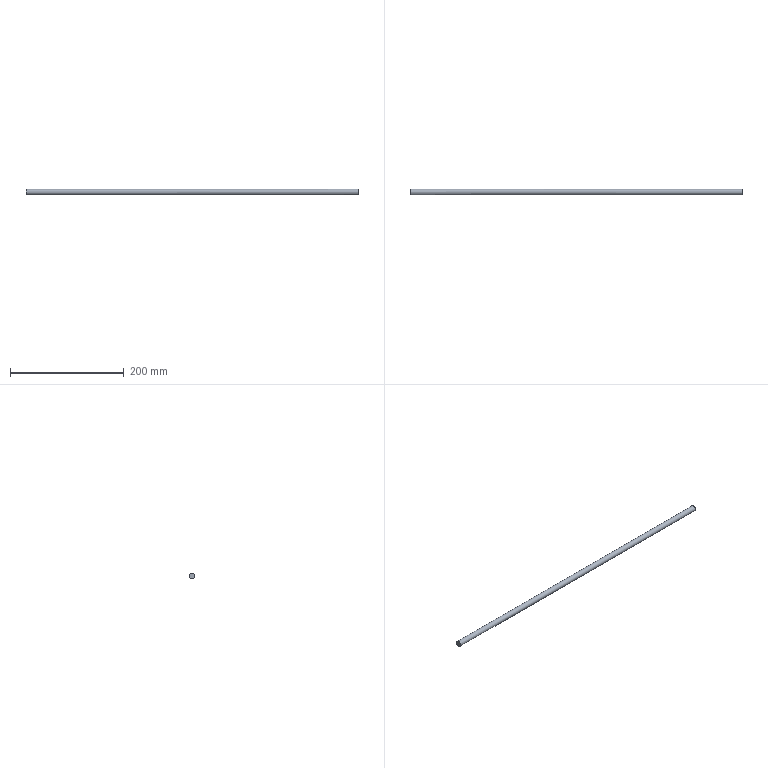Part | NX | features solid 2 | 1 solid | 3 faces | box 585 x 10 x 10 mm | volume 45946 mm3 | plane 2 | cylinder 1 | commonest cylinder face diameters 10 x1
STEP:
#1=CARTESIAN_POINT('',(-312.,-112.5,-292.));
#2=VERTEX_POINT('',#1);
#3=CARTESIAN_POINT('',(-312.,-107.5,-292.));
#4=DIRECTION('',(-1.,0.,0.));
#5=DIRECTION('',(0.,-1.,0.));
#6=AXIS2_PLACEMENT_3D('',#3,#4,#5);
#7=CIRCLE('',#6,5.);
#8=EDGE_CURVE('',#2,#2,#7,.T.);
#9=ORIENTED_EDGE('',*,*,#8,.F.);
#10=EDGE_LOOP('',(#9));
#11=FACE_BOUND('',#10,.T.);
#12=CARTESIAN_POINT('',(273.,-107.5,-297.));
#13=VERTEX_POINT('',#12);
#14=CARTESIAN_POINT('',(273.,-107.5,-292.));
#15=DIRECTION('',(1.,0.,0.));
#16=DIRECTION('',(0.,0.,-1.));
#17=AXIS2_PLACEMENT_3D('',#14,#15,#16);
#18=CIRCLE('',#17,5.);
#19=EDGE_CURVE('',#13,#13,#18,.T.);
#20=ORIENTED_EDGE('',*,*,#19,.F.);
#21=EDGE_LOOP('',(#20));
#22=FACE_BOUND('',#21,.T.);
#23=CARTESIAN_POINT('',(-411.,-107.5,-292.));
#24=DIRECTION('',(1.,0.,0.));
#25=DIRECTION('',(0.,0.,-1.));
#26=AXIS2_PLACEMENT_3D('',#23,#24,#25);
#27=CYLINDRICAL_SURFACE('',#26,5.);
#28=ADVANCED_FACE('',(#11,#22),#27,.T.);
#29=ORIENTED_EDGE('',*,*,#8,.T.);
#30=EDGE_LOOP('',(#29));
#31=FACE_BOUND('',#30,.T.);
#32=CARTESIAN_POINT('',(-312.,-92.,-137.));
#33=DIRECTION('',(-1.,0.,0.));
#34=DIRECTION('',(0.,1.,0.));
#35=AXIS2_PLACEMENT_3D('',#32,#33,#34);
#36=PLANE('',#35);
#37=ADVANCED_FACE('',(#31),#36,.T.);
#38=ORIENTED_EDGE('',*,*,#19,.T.);
#39=EDGE_LOOP('',(#38));
#40=FACE_BOUND('',#39,.T.);
#41=CARTESIAN_POINT('',(273.,25.,-530.));
#42=DIRECTION('',(1.,0.,0.));
#43=DIRECTION('',(0.,0.,-1.));
#44=AXIS2_PLACEMENT_3D('',#41,#42,#43);
#45=PLANE('',#44);
#46=ADVANCED_FACE('',(#40),#45,.T.);
#47=CLOSED_SHELL('',(#28,#37,#46));
#48=MANIFOLD_SOLID_BREP('',#47);
#49=(LENGTH_UNIT()NAMED_UNIT(*)SI_UNIT(.MILLI.,.METRE.));
#50=UNCERTAINTY_MEASURE_WITH_UNIT(LENGTH_MEASURE(0.00001),#49,'','');
#51=(NAMED_UNIT(*)PLANE_ANGLE_UNIT()SI_UNIT($,.RADIAN.));
#52=(NAMED_UNIT(*)SI_UNIT($,.STERADIAN.)SOLID_ANGLE_UNIT());
#53=(GEOMETRIC_REPRESENTATION_CONTEXT(3)GLOBAL_UNCERTAINTY_ASSIGNED_CONTEXT((#50))GLOBAL_UNIT_ASSIGNED_CONTEXT((#49,#51,#52))REPRESENTATION_CONTEXT('',''));
#54=ADVANCED_BREP_SHAPE_REPRESENTATION('',(#48),#53);